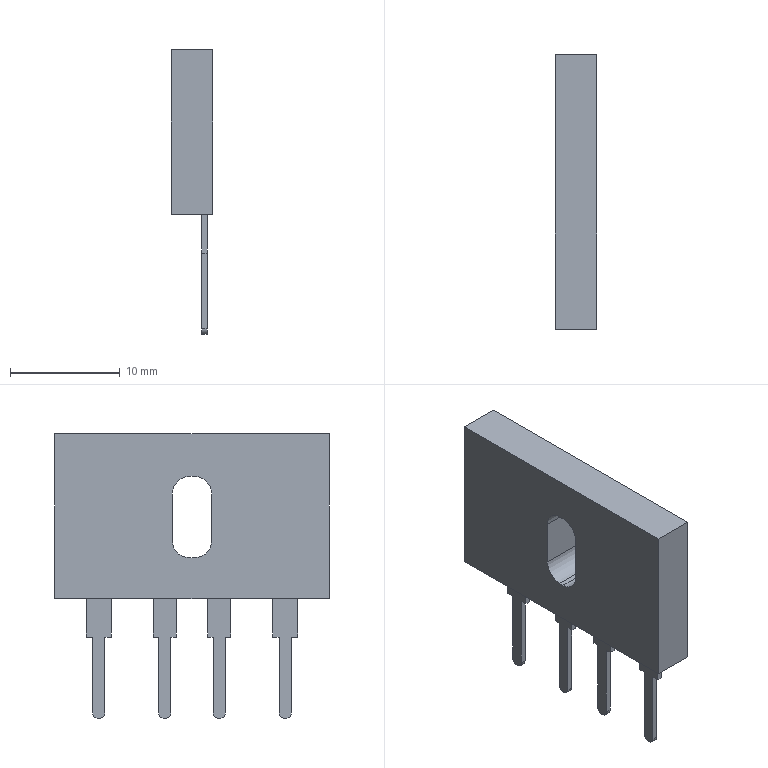Part | STEP file | LRS-150-12_X2_5F00517375-151321 | 1 solid | 58 faces | box 3.75 x 25 x 25.9 mm | volume 1346 mm3 | plane 46 | cylinder 12 | commonest cylinder face diameters 1 x8 3.2 x4